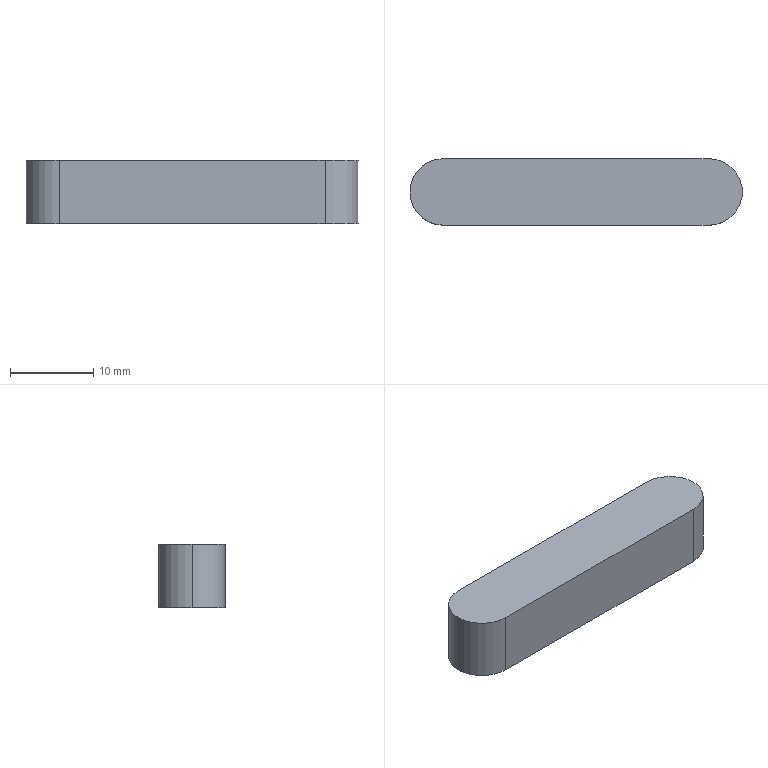Part | STEP file | Keyway 8x40V11_Default<Machined> | 1 solid | 7 faces | box 40 x 8 x 7.7 mm | volume 2358 mm3 | plane 4 | cylinder 3 | commonest cylinder face diameters 8 x3
STEP:
#1=CARTESIAN_POINT('',(0.,0.,0.));
#2=DIRECTION('',(0.,0.,1.));
#3=DIRECTION('',(1.,0.,0.));
#4=AXIS2_PLACEMENT_3D('',#1,#2,#3);
#5=CARTESIAN_POINT('',(-36.,0.,7.7));
#6=VERTEX_POINT('',#5);
#7=CARTESIAN_POINT('',(-32.,-4.,7.7));
#8=VERTEX_POINT('',#7);
#9=CARTESIAN_POINT('',(-32.,0.,7.7));
#10=DIRECTION('',(0.,0.,1.));
#11=DIRECTION('',(1.,0.,0.));
#12=AXIS2_PLACEMENT_3D('',#9,#10,#11);
#13=CIRCLE('',#12,4.);
#14=CARTESIAN_POINT('',(-32.,0.,7.7));
#15=DIRECTION('',(0.,0.,-1.));
#16=DIRECTION('',(-1.,0.,0.));
#17=AXIS2_PLACEMENT_3D('',#14,#15,#16);
#18=CYLINDRICAL_SURFACE('',#17,4.);
#19=CARTESIAN_POINT('',(9.425,0.));
#20=DIRECTION('',(-1.,0.));
#21=VECTOR('',#20,1.);
#22=LINE('',#19,#21);
#23=(GEOMETRIC_REPRESENTATION_CONTEXT(2)PARAMETRIC_REPRESENTATION_CONTEXT()REPRESENTATION_CONTEXT('',''));
#24=DEFINITIONAL_REPRESENTATION('',(#22),#23);
#25=PCURVE('',#18,#24);
#26=CARTESIAN_POINT('',(0.,0.,7.7));
#27=DIRECTION('',(0.,0.,1.));
#28=DIRECTION('',(1.,0.,0.));
#29=AXIS2_PLACEMENT_3D('',#26,#27,#28);
#30=PLANE('',#29);
#31=CARTESIAN_POINT('',(-32.,0.));
#32=DIRECTION('',(1.,0.));
#33=AXIS2_PLACEMENT_2D('',#31,#32);
#34=CIRCLE('',#33,4.);
#35=(GEOMETRIC_REPRESENTATION_CONTEXT(2)PARAMETRIC_REPRESENTATION_CONTEXT()REPRESENTATION_CONTEXT('',''));
#36=DEFINITIONAL_REPRESENTATION('',(#34),#35);
#37=PCURVE('',#30,#36);
#38=SURFACE_CURVE('',#13,(#25,#37),.PCURVE_S1.);
#39=EDGE_CURVE('',#6,#8,#38,.T.);
#40=ORIENTED_EDGE('',*,*,#39,.F.);
#41=CARTESIAN_POINT('',(-36.,0.,0.));
#42=VERTEX_POINT('',#41);
#43=CARTESIAN_POINT('',(-36.,0.,7.7));
#44=DIRECTION('',(0.,0.,-1.));
#45=VECTOR('',#44,1.);
#46=LINE('',#43,#45);
#47=CARTESIAN_POINT('',(6.283,0.));
#48=DIRECTION('',(0.,1.));
#49=VECTOR('',#48,1.);
#50=LINE('',#47,#49);
#51=(GEOMETRIC_REPRESENTATION_CONTEXT(2)PARAMETRIC_REPRESENTATION_CONTEXT()REPRESENTATION_CONTEXT('',''));
#52=DEFINITIONAL_REPRESENTATION('',(#50),#51);
#53=PCURVE('',#18,#52);
#54=CARTESIAN_POINT('',(-32.,0.,7.7));
#55=DIRECTION('',(0.,0.,-1.));
#56=DIRECTION('',(-1.,0.,0.));
#57=AXIS2_PLACEMENT_3D('',#54,#55,#56);
#58=CYLINDRICAL_SURFACE('',#57,4.);
#59=CARTESIAN_POINT('',(0.,0.));
#60=DIRECTION('',(0.,1.));
#61=VECTOR('',#60,1.);
#62=LINE('',#59,#61);
#63=(GEOMETRIC_REPRESENTATION_CONTEXT(2)PARAMETRIC_REPRESENTATION_CONTEXT()REPRESENTATION_CONTEXT('',''));
#64=DEFINITIONAL_REPRESENTATION('',(#62),#63);
#65=PCURVE('',#58,#64);
#66=SURFACE_CURVE('',#46,(#53,#65),.PCURVE_S1.);
#67=EDGE_CURVE('',#6,#42,#66,.T.);
#68=ORIENTED_EDGE('',*,*,#67,.T.);
#69=CARTESIAN_POINT('',(-32.,-4.,0.));
#70=VERTEX_POINT('',#69);
#71=CARTESIAN_POINT('',(-32.,0.,0.));
#72=DIRECTION('',(0.,0.,1.));
#73=DIRECTION('',(1.,0.,0.));
#74=AXIS2_PLACEMENT_3D('',#71,#72,#73);
#75=CIRCLE('',#74,4.);
#76=CARTESIAN_POINT('',(9.425,7.7));
#77=DIRECTION('',(-1.,0.));
#78=VECTOR('',#77,1.);
#79=LINE('',#76,#78);
#80=(GEOMETRIC_REPRESENTATION_CONTEXT(2)PARAMETRIC_REPRESENTATION_CONTEXT()REPRESENTATION_CONTEXT('',''));
#81=DEFINITIONAL_REPRESENTATION('',(#79),#80);
#82=PCURVE('',#18,#81);
#83=CARTESIAN_POINT('',(0.,0.,0.));
#84=DIRECTION('',(0.,0.,1.));
#85=DIRECTION('',(1.,0.,0.));
#86=AXIS2_PLACEMENT_3D('',#83,#84,#85);
#87=PLANE('',#86);
#88=CARTESIAN_POINT('',(-32.,0.));
#89=DIRECTION('',(1.,0.));
#90=AXIS2_PLACEMENT_2D('',#88,#89);
#91=CIRCLE('',#90,4.);
#92=(GEOMETRIC_REPRESENTATION_CONTEXT(2)PARAMETRIC_REPRESENTATION_CONTEXT()REPRESENTATION_CONTEXT('',''));
#93=DEFINITIONAL_REPRESENTATION('',(#91),#92);
#94=PCURVE('',#87,#93);
#95=SURFACE_CURVE('',#75,(#82,#94),.PCURVE_S1.);
#96=EDGE_CURVE('',#42,#70,#95,.T.);
#97=ORIENTED_EDGE('',*,*,#96,.T.);
#98=CARTESIAN_POINT('',(-32.,-4.,7.7));
#99=DIRECTION('',(0.,0.,-1.));
#100=VECTOR('',#99,1.);
#101=LINE('',#98,#100);
#102=CARTESIAN_POINT('',(4.712,0.));
#103=DIRECTION('',(0.,1.));
#104=VECTOR('',#103,1.);
#105=LINE('',#102,#104);
#106=(GEOMETRIC_REPRESENTATION_CONTEXT(2)PARAMETRIC_REPRESENTATION_CONTEXT()REPRESENTATION_CONTEXT('',''));
#107=DEFINITIONAL_REPRESENTATION('',(#105),#106);
#108=PCURVE('',#18,#107);
#109=CARTESIAN_POINT('',(0.,-4.,7.7));
#110=DIRECTION('',(0.,1.,0.));
#111=DIRECTION('',(-1.,0.,0.));
#112=AXIS2_PLACEMENT_3D('',#109,#110,#111);
#113=PLANE('',#112);
#114=CARTESIAN_POINT('',(32.,0.));
#115=DIRECTION('',(0.,-1.));
#116=VECTOR('',#115,1.);
#117=LINE('',#114,#116);
#118=(GEOMETRIC_REPRESENTATION_CONTEXT(2)PARAMETRIC_REPRESENTATION_CONTEXT()REPRESENTATION_CONTEXT('',''));
#119=DEFINITIONAL_REPRESENTATION('',(#117),#118);
#120=PCURVE('',#113,#119);
#121=SURFACE_CURVE('',#101,(#108,#120),.PCURVE_S1.);
#122=EDGE_CURVE('',#8,#70,#121,.T.);
#123=ORIENTED_EDGE('',*,*,#122,.F.);
#124=EDGE_LOOP('',(#40,#68,#97,#123));
#125=FACE_BOUND('',#124,.T.);
#126=ADVANCED_FACE('',(#125),#18,.T.);
#127=CARTESIAN_POINT('',(0.,-4.,0.));
#128=VERTEX_POINT('',#127);
#129=CARTESIAN_POINT('',(0.,4.,0.));
#130=VERTEX_POINT('',#129);
#131=CARTESIAN_POINT('',(0.,0.,0.));
#132=DIRECTION('',(0.,0.,1.));
#133=DIRECTION('',(1.,0.,0.));
#134=AXIS2_PLACEMENT_3D('',#131,#132,#133);
#135=CIRCLE('',#134,4.);
#136=CARTESIAN_POINT('',(0.,0.,7.7));
#137=DIRECTION('',(0.,0.,-1.));
#138=DIRECTION('',(-1.,0.,0.));
#139=AXIS2_PLACEMENT_3D('',#136,#137,#138);
#140=CYLINDRICAL_SURFACE('',#139,4.);
#141=CARTESIAN_POINT('',(9.425,7.7));
#142=DIRECTION('',(-1.,0.));
#143=VECTOR('',#142,1.);
#144=LINE('',#141,#143);
#145=(GEOMETRIC_REPRESENTATION_CONTEXT(2)PARAMETRIC_REPRESENTATION_CONTEXT()REPRESENTATION_CONTEXT('',''));
#146=DEFINITIONAL_REPRESENTATION('',(#144),#145);
#147=PCURVE('',#140,#146);
#148=CARTESIAN_POINT('',(0.,0.));
#149=DIRECTION('',(1.,0.));
#150=AXIS2_PLACEMENT_2D('',#148,#149);
#151=CIRCLE('',#150,4.);
#152=(GEOMETRIC_REPRESENTATION_CONTEXT(2)PARAMETRIC_REPRESENTATION_CONTEXT()REPRESENTATION_CONTEXT('',''));
#153=DEFINITIONAL_REPRESENTATION('',(#151),#152);
#154=PCURVE('',#87,#153);
#155=SURFACE_CURVE('',#135,(#147,#154),.PCURVE_S1.);
#156=EDGE_CURVE('',#128,#130,#155,.T.);
#157=ORIENTED_EDGE('',*,*,#156,.T.);
#158=CARTESIAN_POINT('',(0.,4.,7.7));
#159=VERTEX_POINT('',#158);
#160=CARTESIAN_POINT('',(0.,4.,7.7));
#161=DIRECTION('',(0.,0.,-1.));
#162=VECTOR('',#161,1.);
#163=LINE('',#160,#162);
#164=CARTESIAN_POINT('',(1.571,0.));
#165=DIRECTION('',(0.,1.));
#166=VECTOR('',#165,1.);
#167=LINE('',#164,#166);
#168=(GEOMETRIC_REPRESENTATION_CONTEXT(2)PARAMETRIC_REPRESENTATION_CONTEXT()REPRESENTATION_CONTEXT('',''));
#169=DEFINITIONAL_REPRESENTATION('',(#167),#168);
#170=PCURVE('',#140,#169);
#171=CARTESIAN_POINT('',(0.,4.,7.7));
#172=DIRECTION('',(0.,-1.,0.));
#173=DIRECTION('',(1.,0.,0.));
#174=AXIS2_PLACEMENT_3D('',#171,#172,#173);
#175=PLANE('',#174);
#176=CARTESIAN_POINT('',(0.,0.));
#177=DIRECTION('',(0.,-1.));
#178=VECTOR('',#177,1.);
#179=LINE('',#176,#178);
#180=(GEOMETRIC_REPRESENTATION_CONTEXT(2)PARAMETRIC_REPRESENTATION_CONTEXT()REPRESENTATION_CONTEXT('',''));
#181=DEFINITIONAL_REPRESENTATION('',(#179),#180);
#182=PCURVE('',#175,#181);
#183=SURFACE_CURVE('',#163,(#170,#182),.PCURVE_S1.);
#184=EDGE_CURVE('',#159,#130,#183,.T.);
#185=ORIENTED_EDGE('',*,*,#184,.F.);
#186=CARTESIAN_POINT('',(0.,-4.,7.7));
#187=VERTEX_POINT('',#186);
#188=CARTESIAN_POINT('',(0.,0.,7.7));
#189=DIRECTION('',(0.,0.,1.));
#190=DIRECTION('',(1.,0.,0.));
#191=AXIS2_PLACEMENT_3D('',#188,#189,#190);
#192=CIRCLE('',#191,4.);
#193=CARTESIAN_POINT('',(9.425,0.));
#194=DIRECTION('',(-1.,0.));
#195=VECTOR('',#194,1.);
#196=LINE('',#193,#195);
#197=(GEOMETRIC_REPRESENTATION_CONTEXT(2)PARAMETRIC_REPRESENTATION_CONTEXT()REPRESENTATION_CONTEXT('',''));
#198=DEFINITIONAL_REPRESENTATION('',(#196),#197);
#199=PCURVE('',#140,#198);
#200=CARTESIAN_POINT('',(0.,0.));
#201=DIRECTION('',(1.,0.));
#202=AXIS2_PLACEMENT_2D('',#200,#201);
#203=CIRCLE('',#202,4.);
#204=(GEOMETRIC_REPRESENTATION_CONTEXT(2)PARAMETRIC_REPRESENTATION_CONTEXT()REPRESENTATION_CONTEXT('',''));
#205=DEFINITIONAL_REPRESENTATION('',(#203),#204);
#206=PCURVE('',#30,#205);
#207=SURFACE_CURVE('',#192,(#199,#206),.PCURVE_S1.);
#208=EDGE_CURVE('',#187,#159,#207,.T.);
#209=ORIENTED_EDGE('',*,*,#208,.F.);
#210=CARTESIAN_POINT('',(0.,-4.,7.7));
#211=DIRECTION('',(0.,0.,-1.));
#212=VECTOR('',#211,1.);
#213=LINE('',#210,#212);
#214=CARTESIAN_POINT('',(4.712,0.));
#215=DIRECTION('',(0.,1.));
#216=VECTOR('',#215,1.);
#217=LINE('',#214,#216);
#218=(GEOMETRIC_REPRESENTATION_CONTEXT(2)PARAMETRIC_REPRESENTATION_CONTEXT()REPRESENTATION_CONTEXT('',''));
#219=DEFINITIONAL_REPRESENTATION('',(#217),#218);
#220=PCURVE('',#140,#219);
#221=CARTESIAN_POINT('',(0.,0.));
#222=DIRECTION('',(0.,-1.));
#223=VECTOR('',#222,1.);
#224=LINE('',#221,#223);
#225=(GEOMETRIC_REPRESENTATION_CONTEXT(2)PARAMETRIC_REPRESENTATION_CONTEXT()REPRESENTATION_CONTEXT('',''));
#226=DEFINITIONAL_REPRESENTATION('',(#224),#225);
#227=PCURVE('',#113,#226);
#228=SURFACE_CURVE('',#213,(#220,#227),.PCURVE_S1.);
#229=EDGE_CURVE('',#187,#128,#228,.T.);
#230=ORIENTED_EDGE('',*,*,#229,.T.);
#231=EDGE_LOOP('',(#157,#185,#209,#230));
#232=FACE_BOUND('',#231,.T.);
#233=ADVANCED_FACE('',(#232),#140,.T.);
#234=CARTESIAN_POINT('',(-32.,4.,0.));
#235=VERTEX_POINT('',#234);
#236=CARTESIAN_POINT('',(0.,4.,0.));
#237=DIRECTION('',(-1.,0.,0.));
#238=VECTOR('',#237,1.);
#239=LINE('',#236,#238);
#240=CARTESIAN_POINT('',(0.,-7.7));
#241=DIRECTION('',(-1.,0.));
#242=VECTOR('',#241,1.);
#243=LINE('',#240,#242);
#244=(GEOMETRIC_REPRESENTATION_CONTEXT(2)PARAMETRIC_REPRESENTATION_CONTEXT()REPRESENTATION_CONTEXT('',''));
#245=DEFINITIONAL_REPRESENTATION('',(#243),#244);
#246=PCURVE('',#175,#245);
#247=CARTESIAN_POINT('',(0.,4.));
#248=DIRECTION('',(-1.,0.));
#249=VECTOR('',#248,1.);
#250=LINE('',#247,#249);
#251=(GEOMETRIC_REPRESENTATION_CONTEXT(2)PARAMETRIC_REPRESENTATION_CONTEXT()REPRESENTATION_CONTEXT('',''));
#252=DEFINITIONAL_REPRESENTATION('',(#250),#251);
#253=PCURVE('',#87,#252);
#254=SURFACE_CURVE('',#239,(#246,#253),.PCURVE_S1.);
#255=EDGE_CURVE('',#130,#235,#254,.T.);
#256=ORIENTED_EDGE('',*,*,#255,.T.);
#257=CARTESIAN_POINT('',(-32.,4.,7.7));
#258=VERTEX_POINT('',#257);
#259=CARTESIAN_POINT('',(-32.,4.,7.7));
#260=DIRECTION('',(0.,0.,-1.));
#261=VECTOR('',#260,1.);
#262=LINE('',#259,#261);
#263=CARTESIAN_POINT('',(-32.,0.));
#264=DIRECTION('',(0.,-1.));
#265=VECTOR('',#264,1.);
#266=LINE('',#263,#265);
#267=(GEOMETRIC_REPRESENTATION_CONTEXT(2)PARAMETRIC_REPRESENTATION_CONTEXT()REPRESENTATION_CONTEXT('',''));
#268=DEFINITIONAL_REPRESENTATION('',(#266),#267);
#269=PCURVE('',#175,#268);
#270=CARTESIAN_POINT('',(1.571,0.));
#271=DIRECTION('',(0.,1.));
#272=VECTOR('',#271,1.);
#273=LINE('',#270,#272);
#274=(GEOMETRIC_REPRESENTATION_CONTEXT(2)PARAMETRIC_REPRESENTATION_CONTEXT()REPRESENTATION_CONTEXT('',''));
#275=DEFINITIONAL_REPRESENTATION('',(#273),#274);
#276=PCURVE('',#58,#275);
#277=SURFACE_CURVE('',#262,(#269,#276),.PCURVE_S1.);
#278=EDGE_CURVE('',#258,#235,#277,.T.);
#279=ORIENTED_EDGE('',*,*,#278,.F.);
#280=CARTESIAN_POINT('',(0.,4.,7.7));
#281=DIRECTION('',(-1.,0.,0.));
#282=VECTOR('',#281,1.);
#283=LINE('',#280,#282);
#284=CARTESIAN_POINT('',(0.,0.));
#285=DIRECTION('',(-1.,0.));
#286=VECTOR('',#285,1.);
#287=LINE('',#284,#286);
#288=(GEOMETRIC_REPRESENTATION_CONTEXT(2)PARAMETRIC_REPRESENTATION_CONTEXT()REPRESENTATION_CONTEXT('',''));
#289=DEFINITIONAL_REPRESENTATION('',(#287),#288);
#290=PCURVE('',#175,#289);
#291=CARTESIAN_POINT('',(0.,4.));
#292=DIRECTION('',(-1.,0.));
#293=VECTOR('',#292,1.);
#294=LINE('',#291,#293);
#295=(GEOMETRIC_REPRESENTATION_CONTEXT(2)PARAMETRIC_REPRESENTATION_CONTEXT()REPRESENTATION_CONTEXT('',''));
#296=DEFINITIONAL_REPRESENTATION('',(#294),#295);
#297=PCURVE('',#30,#296);
#298=SURFACE_CURVE('',#283,(#290,#297),.PCURVE_S1.);
#299=EDGE_CURVE('',#159,#258,#298,.T.);
#300=ORIENTED_EDGE('',*,*,#299,.F.);
#301=ORIENTED_EDGE('',*,*,#184,.T.);
#302=EDGE_LOOP('',(#256,#279,#300,#301));
#303=FACE_BOUND('',#302,.T.);
#304=ADVANCED_FACE('',(#303),#175,.F.);
#305=ORIENTED_EDGE('',*,*,#67,.F.);
#306=CARTESIAN_POINT('',(-32.,0.,7.7));
#307=DIRECTION('',(0.,0.,1.));
#308=DIRECTION('',(1.,0.,0.));
#309=AXIS2_PLACEMENT_3D('',#306,#307,#308);
#310=CIRCLE('',#309,4.);
#311=CARTESIAN_POINT('',(3.142,0.));
#312=DIRECTION('',(-1.,0.));
#313=VECTOR('',#312,1.);
#314=LINE('',#311,#313);
#315=(GEOMETRIC_REPRESENTATION_CONTEXT(2)PARAMETRIC_REPRESENTATION_CONTEXT()REPRESENTATION_CONTEXT('',''));
#316=DEFINITIONAL_REPRESENTATION('',(#314),#315);
#317=PCURVE('',#58,#316);
#318=CARTESIAN_POINT('',(-32.,0.));
#319=DIRECTION('',(1.,0.));
#320=AXIS2_PLACEMENT_2D('',#318,#319);
#321=CIRCLE('',#320,4.);
#322=(GEOMETRIC_REPRESENTATION_CONTEXT(2)PARAMETRIC_REPRESENTATION_CONTEXT()REPRESENTATION_CONTEXT('',''));
#323=DEFINITIONAL_REPRESENTATION('',(#321),#322);
#324=PCURVE('',#30,#323);
#325=SURFACE_CURVE('',#310,(#317,#324),.PCURVE_S1.);
#326=EDGE_CURVE('',#258,#6,#325,.T.);
#327=ORIENTED_EDGE('',*,*,#326,.F.);
#328=ORIENTED_EDGE('',*,*,#278,.T.);
#329=CARTESIAN_POINT('',(-32.,0.,0.));
#330=DIRECTION('',(0.,0.,1.));
#331=DIRECTION('',(1.,0.,0.));
#332=AXIS2_PLACEMENT_3D('',#329,#330,#331);
#333=CIRCLE('',#332,4.);
#334=CARTESIAN_POINT('',(3.142,7.7));
#335=DIRECTION('',(-1.,0.));
#336=VECTOR('',#335,1.);
#337=LINE('',#334,#336);
#338=(GEOMETRIC_REPRESENTATION_CONTEXT(2)PARAMETRIC_REPRESENTATION_CONTEXT()REPRESENTATION_CONTEXT('',''));
#339=DEFINITIONAL_REPRESENTATION('',(#337),#338);
#340=PCURVE('',#58,#339);
#341=CARTESIAN_POINT('',(-32.,0.));
#342=DIRECTION('',(1.,0.));
#343=AXIS2_PLACEMENT_2D('',#341,#342);
#344=CIRCLE('',#343,4.);
#345=(GEOMETRIC_REPRESENTATION_CONTEXT(2)PARAMETRIC_REPRESENTATION_CONTEXT()REPRESENTATION_CONTEXT('',''));
#346=DEFINITIONAL_REPRESENTATION('',(#344),#345);
#347=PCURVE('',#87,#346);
#348=SURFACE_CURVE('',#333,(#340,#347),.PCURVE_S1.);
#349=EDGE_CURVE('',#235,#42,#348,.T.);
#350=ORIENTED_EDGE('',*,*,#349,.T.);
#351=EDGE_LOOP('',(#305,#327,#328,#350));
#352=FACE_BOUND('',#351,.T.);
#353=ADVANCED_FACE('',(#352),#58,.T.);
#354=CARTESIAN_POINT('',(0.,-4.,0.));
#355=DIRECTION('',(1.,0.,0.));
#356=VECTOR('',#355,1.);
#357=LINE('',#354,#356);
#358=CARTESIAN_POINT('',(0.,-7.7));
#359=DIRECTION('',(-1.,0.));
#360=VECTOR('',#359,1.);
#361=LINE('',#358,#360);
#362=(GEOMETRIC_REPRESENTATION_CONTEXT(2)PARAMETRIC_REPRESENTATION_CONTEXT()REPRESENTATION_CONTEXT('',''));
#363=DEFINITIONAL_REPRESENTATION('',(#361),#362);
#364=PCURVE('',#113,#363);
#365=CARTESIAN_POINT('',(0.,-4.));
#366=DIRECTION('',(1.,0.));
#367=VECTOR('',#366,1.);
#368=LINE('',#365,#367);
#369=(GEOMETRIC_REPRESENTATION_CONTEXT(2)PARAMETRIC_REPRESENTATION_CONTEXT()REPRESENTATION_CONTEXT('',''));
#370=DEFINITIONAL_REPRESENTATION('',(#368),#369);
#371=PCURVE('',#87,#370);
#372=SURFACE_CURVE('',#357,(#364,#371),.PCURVE_S1.);
#373=EDGE_CURVE('',#70,#128,#372,.T.);
#374=ORIENTED_EDGE('',*,*,#373,.T.);
#375=ORIENTED_EDGE('',*,*,#229,.F.);
#376=CARTESIAN_POINT('',(0.,-4.,7.7));
#377=DIRECTION('',(1.,0.,0.));
#378=VECTOR('',#377,1.);
#379=LINE('',#376,#378);
#380=CARTESIAN_POINT('',(0.,0.));
#381=DIRECTION('',(-1.,0.));
#382=VECTOR('',#381,1.);
#383=LINE('',#380,#382);
#384=(GEOMETRIC_REPRESENTATION_CONTEXT(2)PARAMETRIC_REPRESENTATION_CONTEXT()REPRESENTATION_CONTEXT('',''));
#385=DEFINITIONAL_REPRESENTATION('',(#383),#384);
#386=PCURVE('',#113,#385);
#387=CARTESIAN_POINT('',(0.,-4.));
#388=DIRECTION('',(1.,0.));
#389=VECTOR('',#388,1.);
#390=LINE('',#387,#389);
#391=(GEOMETRIC_REPRESENTATION_CONTEXT(2)PARAMETRIC_REPRESENTATION_CONTEXT()REPRESENTATION_CONTEXT('',''));
#392=DEFINITIONAL_REPRESENTATION('',(#390),#391);
#393=PCURVE('',#30,#392);
#394=SURFACE_CURVE('',#379,(#386,#393),.PCURVE_S1.);
#395=EDGE_CURVE('',#8,#187,#394,.T.);
#396=ORIENTED_EDGE('',*,*,#395,.F.);
#397=ORIENTED_EDGE('',*,*,#122,.T.);
#398=EDGE_LOOP('',(#374,#375,#396,#397));
#399=FACE_BOUND('',#398,.T.);
#400=ADVANCED_FACE('',(#399),#113,.F.);
#401=ORIENTED_EDGE('',*,*,#208,.T.);
#402=ORIENTED_EDGE('',*,*,#299,.T.);
#403=ORIENTED_EDGE('',*,*,#326,.T.);
#404=ORIENTED_EDGE('',*,*,#39,.T.);
#405=ORIENTED_EDGE('',*,*,#395,.T.);
#406=EDGE_LOOP('',(#401,#402,#403,#404,#405));
#407=FACE_BOUND('',#406,.T.);
#408=ADVANCED_FACE('',(#407),#30,.T.);
#409=ORIENTED_EDGE('',*,*,#156,.F.);
#410=ORIENTED_EDGE('',*,*,#373,.F.);
#411=ORIENTED_EDGE('',*,*,#96,.F.);
#412=ORIENTED_EDGE('',*,*,#349,.F.);
#413=ORIENTED_EDGE('',*,*,#255,.F.);
#414=EDGE_LOOP('',(#409,#410,#411,#412,#413));
#415=FACE_BOUND('',#414,.T.);
#416=ADVANCED_FACE('',(#415),#87,.F.);
#417=CLOSED_SHELL('',(#126,#233,#304,#353,#400,#408,#416));
#418=MANIFOLD_SOLID_BREP('',#417);
#419=(LENGTH_UNIT()NAMED_UNIT(*)SI_UNIT(.MILLI.,.METRE.));
#420=UNCERTAINTY_MEASURE_WITH_UNIT(LENGTH_MEASURE(0.0000001),#419,'','');
#421=(NAMED_UNIT(*)PLANE_ANGLE_UNIT()SI_UNIT($,.RADIAN.));
#422=(NAMED_UNIT(*)SI_UNIT($,.STERADIAN.)SOLID_ANGLE_UNIT());
#423=(GEOMETRIC_REPRESENTATION_CONTEXT(3)GLOBAL_UNCERTAINTY_ASSIGNED_CONTEXT((#420))GLOBAL_UNIT_ASSIGNED_CONTEXT((#419,#421,#422))REPRESENTATION_CONTEXT('',''));
#424=ADVANCED_BREP_SHAPE_REPRESENTATION('',(#4,#418),#423);